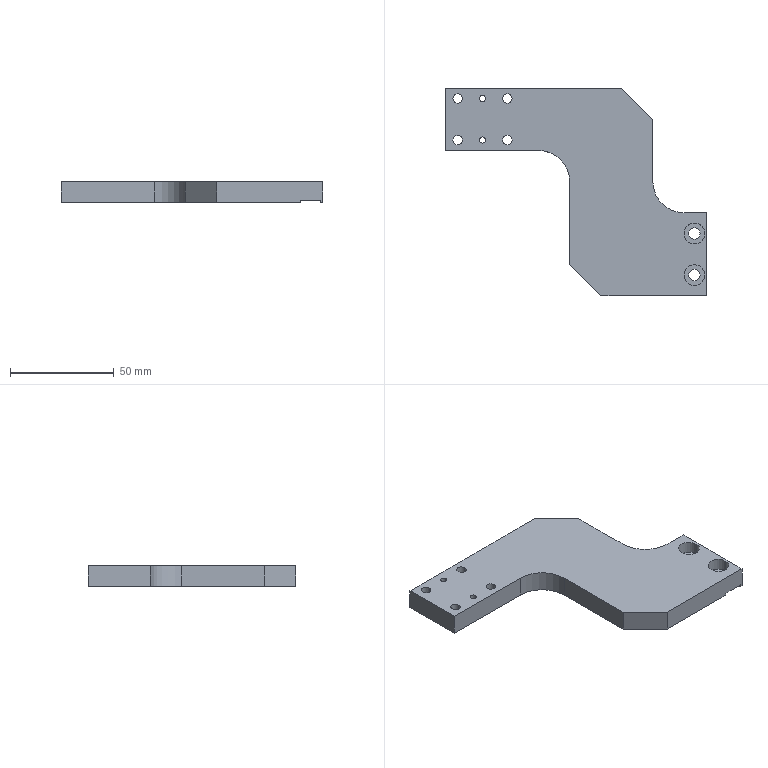Part | STEP file | PN_0076 Mount electronic clip suction nozzle connecting plate | 1 solid | 52 faces | box 126 x 100 x 10 mm | volume 64254 mm3 | cylinder 30 | plane 22 | commonest cylinder face diameters 4.5 x8 8 x8 3 x4 5.5 x4 10 x4 30 x2